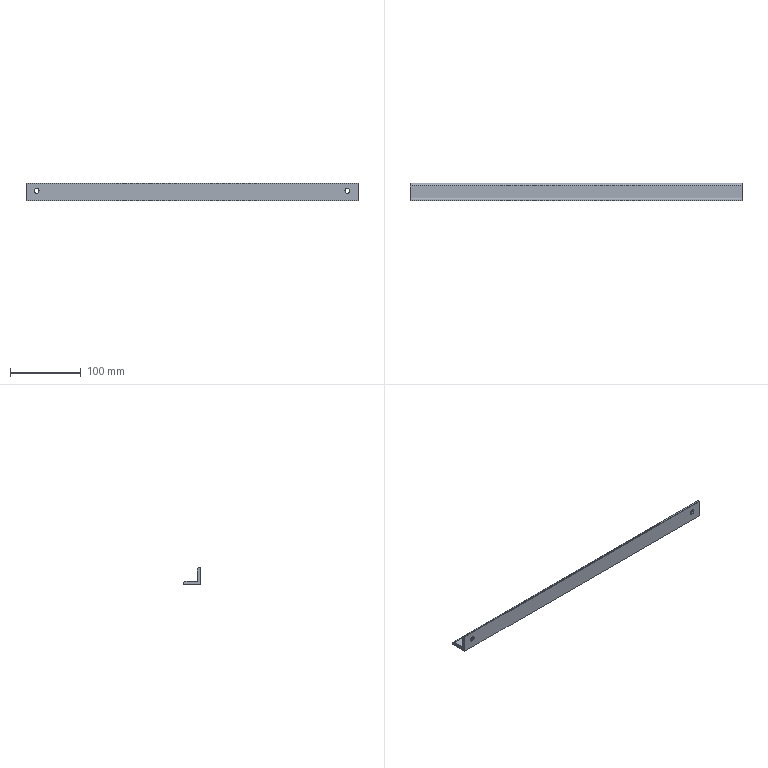Part | NX | 1 solid | 18 faces | box 470 x 25 x 25 mm | volume 101967 mm3 | plane 8 | cylinder 6 | cone 4 | commonest cylinder face diameters 7 x4 8 x2
STEP:
#1=CARTESIAN_POINT('',(-260.,12.5,-11.5));
#2=VERTEX_POINT('',#1);
#3=CARTESIAN_POINT('',(-260.,12.5,-12.5));
#4=VERTEX_POINT('',#3);
#5=CARTESIAN_POINT('',(-260.,12.5,0.));
#6=DIRECTION('',(0.,0.,-1.));
#7=VECTOR('',#6,1000.);
#8=LINE('',#5,#7);
#9=EDGE_CURVE('',#2,#4,#8,.T.);
#10=ORIENTED_EDGE('',*,*,#9,.T.);
#11=CARTESIAN_POINT('',(-260.,-12.5,-12.5));
#12=VERTEX_POINT('',#11);
#13=CARTESIAN_POINT('',(-260.,0.,-12.5));
#14=DIRECTION('',(0.,-1.,0.));
#15=VECTOR('',#14,1000.);
#16=LINE('',#13,#15);
#17=EDGE_CURVE('',#4,#12,#16,.T.);
#18=ORIENTED_EDGE('',*,*,#17,.T.);
#19=CARTESIAN_POINT('',(-260.,-12.5,12.5));
#20=VERTEX_POINT('',#19);
#21=CARTESIAN_POINT('',(-260.,-12.5,0.));
#22=DIRECTION('',(0.,0.,1.));
#23=VECTOR('',#22,1000.);
#24=LINE('',#21,#23);
#25=EDGE_CURVE('',#12,#20,#24,.T.);
#26=ORIENTED_EDGE('',*,*,#25,.T.);
#27=CARTESIAN_POINT('',(-260.,-11.5,12.5));
#28=VERTEX_POINT('',#27);
#29=CARTESIAN_POINT('',(-260.,0.,12.5));
#30=DIRECTION('',(0.,1.,0.));
#31=VECTOR('',#30,1000.);
#32=LINE('',#29,#31);
#33=EDGE_CURVE('',#20,#28,#32,.T.);
#34=ORIENTED_EDGE('',*,*,#33,.T.);
#35=CARTESIAN_POINT('',(-260.,-7.5,8.5));
#36=VERTEX_POINT('',#35);
#37=CARTESIAN_POINT('',(-260.,-11.5,8.5));
#38=DIRECTION('',(1.,0.,0.));
#39=DIRECTION('',(0.,0.,-1.));
#40=AXIS2_PLACEMENT_3D('',#37,#38,#39);
#41=CIRCLE('',#40,4.);
#42=EDGE_CURVE('',#36,#28,#41,.T.);
#43=ORIENTED_EDGE('',*,*,#42,.F.);
#44=CARTESIAN_POINT('',(-260.,-7.5,-7.5));
#45=VERTEX_POINT('',#44);
#46=CARTESIAN_POINT('',(-260.,-7.5,0.));
#47=DIRECTION('',(0.,0.,-1.));
#48=VECTOR('',#47,1000.);
#49=LINE('',#46,#48);
#50=EDGE_CURVE('',#36,#45,#49,.T.);
#51=ORIENTED_EDGE('',*,*,#50,.T.);
#52=CARTESIAN_POINT('',(-260.,8.5,-7.5));
#53=VERTEX_POINT('',#52);
#54=CARTESIAN_POINT('',(-260.,0.,-7.5));
#55=DIRECTION('',(0.,1.,0.));
#56=VECTOR('',#55,1000.);
#57=LINE('',#54,#56);
#58=EDGE_CURVE('',#45,#53,#57,.T.);
#59=ORIENTED_EDGE('',*,*,#58,.T.);
#60=CARTESIAN_POINT('',(-260.,8.5,-11.5));
#61=DIRECTION('',(1.,0.,0.));
#62=DIRECTION('',(0.,0.,-1.));
#63=AXIS2_PLACEMENT_3D('',#60,#61,#62);
#64=CIRCLE('',#63,4.);
#65=EDGE_CURVE('',#2,#53,#64,.T.);
#66=ORIENTED_EDGE('',*,*,#65,.F.);
#67=EDGE_LOOP('',(#10,#18,#26,#34,#43,#51,#59,#66));
#68=FACE_BOUND('',#67,.T.);
#69=CARTESIAN_POINT('',(-260.,0.,0.));
#70=DIRECTION('',(1.,0.,0.));
#71=DIRECTION('',(0.,1.,0.));
#72=AXIS2_PLACEMENT_3D('',#69,#70,#71);
#73=PLANE('',#72);
#74=ADVANCED_FACE('',(#68),#73,.F.);
#75=ORIENTED_EDGE('',*,*,#9,.F.);
#76=CARTESIAN_POINT('',(210.,12.5,-11.5));
#77=VERTEX_POINT('',#76);
#78=CARTESIAN_POINT('',(-260.,12.5,-11.5));
#79=DIRECTION('',(1.,0.,0.));
#80=VECTOR('',#79,1000.);
#81=LINE('',#78,#80);
#82=EDGE_CURVE('',#2,#77,#81,.T.);
#83=ORIENTED_EDGE('',*,*,#82,.T.);
#84=CARTESIAN_POINT('',(210.,12.5,-12.5));
#85=VERTEX_POINT('',#84);
#86=CARTESIAN_POINT('',(210.,12.5,0.));
#87=DIRECTION('',(0.,0.,-1.));
#88=VECTOR('',#87,1000.);
#89=LINE('',#86,#88);
#90=EDGE_CURVE('',#77,#85,#89,.T.);
#91=ORIENTED_EDGE('',*,*,#90,.T.);
#92=CARTESIAN_POINT('',(0.,12.5,-12.5));
#93=DIRECTION('',(-1.,0.,0.));
#94=VECTOR('',#93,1000.);
#95=LINE('',#92,#94);
#96=EDGE_CURVE('',#85,#4,#95,.T.);
#97=ORIENTED_EDGE('',*,*,#96,.T.);
#98=EDGE_LOOP('',(#75,#83,#91,#97));
#99=FACE_BOUND('',#98,.T.);
#100=CARTESIAN_POINT('',(-260.,12.5,-12.5));
#101=DIRECTION('',(0.,1.,0.));
#102=DIRECTION('',(1.,0.,0.));
#103=AXIS2_PLACEMENT_3D('',#100,#101,#102);
#104=PLANE('',#103);
#105=ADVANCED_FACE('',(#99),#104,.T.);
#106=ORIENTED_EDGE('',*,*,#17,.F.);
#107=ORIENTED_EDGE('',*,*,#96,.F.);
#108=CARTESIAN_POINT('',(210.,-12.5,-12.5));
#109=VERTEX_POINT('',#108);
#110=CARTESIAN_POINT('',(210.,0.,-12.5));
#111=DIRECTION('',(0.,-1.,0.));
#112=VECTOR('',#111,1000.);
#113=LINE('',#110,#112);
#114=EDGE_CURVE('',#85,#109,#113,.T.);
#115=ORIENTED_EDGE('',*,*,#114,.T.);
#116=CARTESIAN_POINT('',(0.,-12.5,-12.5));
#117=DIRECTION('',(-1.,0.,0.));
#118=VECTOR('',#117,1000.);
#119=LINE('',#116,#118);
#120=EDGE_CURVE('',#109,#12,#119,.T.);
#121=ORIENTED_EDGE('',*,*,#120,.T.);
#122=EDGE_LOOP('',(#106,#107,#115,#121));
#123=FACE_BOUND('',#122,.T.);
#124=CARTESIAN_POINT('',(-260.,-12.5,-12.5));
#125=DIRECTION('',(0.,0.,-1.));
#126=DIRECTION('',(0.,-1.,0.));
#127=AXIS2_PLACEMENT_3D('',#124,#125,#126);
#128=PLANE('',#127);
#129=ADVANCED_FACE('',(#123),#128,.T.);
#130=ORIENTED_EDGE('',*,*,#25,.F.);
#131=ORIENTED_EDGE('',*,*,#120,.F.);
#132=CARTESIAN_POINT('',(210.,-12.5,12.5));
#133=VERTEX_POINT('',#132);
#134=CARTESIAN_POINT('',(210.,-12.5,0.));
#135=DIRECTION('',(0.,0.,1.));
#136=VECTOR('',#135,1000.);
#137=LINE('',#134,#136);
#138=EDGE_CURVE('',#109,#133,#137,.T.);
#139=ORIENTED_EDGE('',*,*,#138,.T.);
#140=CARTESIAN_POINT('',(0.,-12.5,12.5));
#141=DIRECTION('',(-1.,0.,0.));
#142=VECTOR('',#141,1000.);
#143=LINE('',#140,#142);
#144=EDGE_CURVE('',#133,#20,#143,.T.);
#145=ORIENTED_EDGE('',*,*,#144,.T.);
#146=EDGE_LOOP('',(#130,#131,#139,#145));
#147=FACE_BOUND('',#146,.T.);
#148=CARTESIAN_POINT('',(-248.5,-12.5,1.5));
#149=VERTEX_POINT('',#148);
#150=CARTESIAN_POINT('',(-241.5,-12.5,1.5));
#151=VERTEX_POINT('',#150);
#152=CARTESIAN_POINT('',(-245.,-12.5,1.5));
#153=DIRECTION('',(0.,-1.,0.));
#154=DIRECTION('',(1.,0.,0.));
#155=AXIS2_PLACEMENT_3D('',#152,#153,#154);
#156=CIRCLE('',#155,3.5);
#157=EDGE_CURVE('',#149,#151,#156,.T.);
#158=ORIENTED_EDGE('',*,*,#157,.F.);
#159=CARTESIAN_POINT('',(-245.,-12.5,1.5));
#160=DIRECTION('',(0.,-1.,0.));
#161=DIRECTION('',(1.,0.,0.));
#162=AXIS2_PLACEMENT_3D('',#159,#160,#161);
#163=CIRCLE('',#162,3.5);
#164=EDGE_CURVE('',#151,#149,#163,.T.);
#165=ORIENTED_EDGE('',*,*,#164,.F.);
#166=EDGE_LOOP('',(#158,#165));
#167=FACE_BOUND('',#166,.T.);
#168=CARTESIAN_POINT('',(198.5,-12.5,1.5));
#169=VERTEX_POINT('',#168);
#170=CARTESIAN_POINT('',(191.5,-12.5,1.5));
#171=VERTEX_POINT('',#170);
#172=CARTESIAN_POINT('',(195.,-12.5,1.5));
#173=DIRECTION('',(0.,-1.,0.));
#174=DIRECTION('',(1.,0.,0.));
#175=AXIS2_PLACEMENT_3D('',#172,#173,#174);
#176=CIRCLE('',#175,3.5);
#177=EDGE_CURVE('',#169,#171,#176,.T.);
#178=ORIENTED_EDGE('',*,*,#177,.F.);
#179=CARTESIAN_POINT('',(195.,-12.5,1.5));
#180=DIRECTION('',(0.,-1.,0.));
#181=DIRECTION('',(1.,0.,0.));
#182=AXIS2_PLACEMENT_3D('',#179,#180,#181);
#183=CIRCLE('',#182,3.5);
#184=EDGE_CURVE('',#171,#169,#183,.T.);
#185=ORIENTED_EDGE('',*,*,#184,.F.);
#186=EDGE_LOOP('',(#178,#185));
#187=FACE_BOUND('',#186,.T.);
#188=CARTESIAN_POINT('',(-260.,-12.5,12.5));
#189=DIRECTION('',(0.,-1.,0.));
#190=DIRECTION('',(0.,0.,-1.));
#191=AXIS2_PLACEMENT_3D('',#188,#189,#190);
#192=PLANE('',#191);
#193=ADVANCED_FACE('',(#147,#167,#187),#192,.T.);
#194=ORIENTED_EDGE('',*,*,#33,.F.);
#195=ORIENTED_EDGE('',*,*,#144,.F.);
#196=CARTESIAN_POINT('',(210.,-11.5,12.5));
#197=VERTEX_POINT('',#196);
#198=CARTESIAN_POINT('',(210.,0.,12.5));
#199=DIRECTION('',(0.,1.,0.));
#200=VECTOR('',#199,1000.);
#201=LINE('',#198,#200);
#202=EDGE_CURVE('',#133,#197,#201,.T.);
#203=ORIENTED_EDGE('',*,*,#202,.T.);
#204=CARTESIAN_POINT('',(260.,-11.5,12.5));
#205=DIRECTION('',(-1.,0.,0.));
#206=VECTOR('',#205,1000.);
#207=LINE('',#204,#206);
#208=EDGE_CURVE('',#197,#28,#207,.T.);
#209=ORIENTED_EDGE('',*,*,#208,.T.);
#210=EDGE_LOOP('',(#194,#195,#203,#209));
#211=FACE_BOUND('',#210,.T.);
#212=CARTESIAN_POINT('',(-260.,-11.5,12.5));
#213=DIRECTION('',(0.,0.,1.));
#214=DIRECTION('',(1.,0.,0.));
#215=AXIS2_PLACEMENT_3D('',#212,#213,#214);
#216=PLANE('',#215);
#217=ADVANCED_FACE('',(#211),#216,.T.);
#218=ORIENTED_EDGE('',*,*,#42,.T.);
#219=ORIENTED_EDGE('',*,*,#208,.F.);
#220=CARTESIAN_POINT('',(210.,-7.5,8.5));
#221=VERTEX_POINT('',#220);
#222=CARTESIAN_POINT('',(210.,-11.5,8.5));
#223=DIRECTION('',(1.,0.,0.));
#224=DIRECTION('',(0.,0.,-1.));
#225=AXIS2_PLACEMENT_3D('',#222,#223,#224);
#226=CIRCLE('',#225,4.);
#227=EDGE_CURVE('',#221,#197,#226,.T.);
#228=ORIENTED_EDGE('',*,*,#227,.F.);
#229=CARTESIAN_POINT('',(-260.,-7.5,8.5));
#230=DIRECTION('',(1.,0.,0.));
#231=VECTOR('',#230,1000.);
#232=LINE('',#229,#231);
#233=EDGE_CURVE('',#36,#221,#232,.T.);
#234=ORIENTED_EDGE('',*,*,#233,.F.);
#235=EDGE_LOOP('',(#218,#219,#228,#234));
#236=FACE_BOUND('',#235,.T.);
#237=CARTESIAN_POINT('',(-260.,-11.5,8.5));
#238=DIRECTION('',(1.,0.,0.));
#239=DIRECTION('',(0.,0.,-1.));
#240=AXIS2_PLACEMENT_3D('',#237,#238,#239);
#241=CYLINDRICAL_SURFACE('',#240,4.);
#242=ADVANCED_FACE('',(#236),#241,.T.);
#243=ORIENTED_EDGE('',*,*,#50,.F.);
#244=ORIENTED_EDGE('',*,*,#233,.T.);
#245=CARTESIAN_POINT('',(210.,-7.5,-7.5));
#246=VERTEX_POINT('',#245);
#247=CARTESIAN_POINT('',(210.,-7.5,0.));
#248=DIRECTION('',(0.,0.,-1.));
#249=VECTOR('',#248,1000.);
#250=LINE('',#247,#249);
#251=EDGE_CURVE('',#221,#246,#250,.T.);
#252=ORIENTED_EDGE('',*,*,#251,.T.);
#253=CARTESIAN_POINT('',(0.,-7.5,-7.5));
#254=DIRECTION('',(-1.,0.,0.));
#255=VECTOR('',#254,1000.);
#256=LINE('',#253,#255);
#257=EDGE_CURVE('',#246,#45,#256,.T.);
#258=ORIENTED_EDGE('',*,*,#257,.T.);
#259=EDGE_LOOP('',(#243,#244,#252,#258));
#260=FACE_BOUND('',#259,.T.);
#261=CARTESIAN_POINT('',(-239.,-7.5,1.5));
#262=VERTEX_POINT('',#261);
#263=CARTESIAN_POINT('',(-251.,-7.5,1.5));
#264=VERTEX_POINT('',#263);
#265=CARTESIAN_POINT('',(-245.,-7.5,1.5));
#266=DIRECTION('',(0.,1.,0.));
#267=DIRECTION('',(-1.,0.,0.));
#268=AXIS2_PLACEMENT_3D('',#265,#266,#267);
#269=CIRCLE('',#268,6.);
#270=EDGE_CURVE('',#262,#264,#269,.T.);
#271=ORIENTED_EDGE('',*,*,#270,.F.);
#272=CARTESIAN_POINT('',(-245.,-7.5,1.5));
#273=DIRECTION('',(0.,1.,0.));
#274=DIRECTION('',(-1.,0.,0.));
#275=AXIS2_PLACEMENT_3D('',#272,#273,#274);
#276=CIRCLE('',#275,6.);
#277=EDGE_CURVE('',#264,#262,#276,.T.);
#278=ORIENTED_EDGE('',*,*,#277,.F.);
#279=EDGE_LOOP('',(#271,#278));
#280=FACE_BOUND('',#279,.T.);
#281=CARTESIAN_POINT('',(189.,-7.5,1.5));
#282=VERTEX_POINT('',#281);
#283=CARTESIAN_POINT('',(201.,-7.5,1.5));
#284=VERTEX_POINT('',#283);
#285=CARTESIAN_POINT('',(195.,-7.5,1.5));
#286=DIRECTION('',(0.,1.,0.));
#287=DIRECTION('',(-1.,0.,0.));
#288=AXIS2_PLACEMENT_3D('',#285,#286,#287);
#289=CIRCLE('',#288,6.);
#290=EDGE_CURVE('',#282,#284,#289,.T.);
#291=ORIENTED_EDGE('',*,*,#290,.F.);
#292=CARTESIAN_POINT('',(195.,-7.5,1.5));
#293=DIRECTION('',(0.,1.,0.));
#294=DIRECTION('',(-1.,0.,0.));
#295=AXIS2_PLACEMENT_3D('',#292,#293,#294);
#296=CIRCLE('',#295,6.);
#297=EDGE_CURVE('',#284,#282,#296,.T.);
#298=ORIENTED_EDGE('',*,*,#297,.F.);
#299=EDGE_LOOP('',(#291,#298));
#300=FACE_BOUND('',#299,.T.);
#301=CARTESIAN_POINT('',(-260.,-7.5,-7.5));
#302=DIRECTION('',(0.,1.,0.));
#303=DIRECTION('',(1.,0.,0.));
#304=AXIS2_PLACEMENT_3D('',#301,#302,#303);
#305=PLANE('',#304);
#306=ADVANCED_FACE('',(#260,#280,#300),#305,.T.);
#307=ORIENTED_EDGE('',*,*,#58,.F.);
#308=ORIENTED_EDGE('',*,*,#257,.F.);
#309=CARTESIAN_POINT('',(210.,8.5,-7.5));
#310=VERTEX_POINT('',#309);
#311=CARTESIAN_POINT('',(210.,0.,-7.5));
#312=DIRECTION('',(0.,1.,0.));
#313=VECTOR('',#312,1000.);
#314=LINE('',#311,#313);
#315=EDGE_CURVE('',#246,#310,#314,.T.);
#316=ORIENTED_EDGE('',*,*,#315,.T.);
#317=CARTESIAN_POINT('',(260.,8.5,-7.5));
#318=DIRECTION('',(-1.,0.,0.));
#319=VECTOR('',#318,1000.);
#320=LINE('',#317,#319);
#321=EDGE_CURVE('',#310,#53,#320,.T.);
#322=ORIENTED_EDGE('',*,*,#321,.T.);
#323=EDGE_LOOP('',(#307,#308,#316,#322));
#324=FACE_BOUND('',#323,.T.);
#325=CARTESIAN_POINT('',(-260.,8.5,-7.5));
#326=DIRECTION('',(0.,0.,1.));
#327=DIRECTION('',(1.,0.,0.));
#328=AXIS2_PLACEMENT_3D('',#325,#326,#327);
#329=PLANE('',#328);
#330=ADVANCED_FACE('',(#324),#329,.T.);
#331=ORIENTED_EDGE('',*,*,#65,.T.);
#332=ORIENTED_EDGE('',*,*,#321,.F.);
#333=CARTESIAN_POINT('',(210.,8.5,-11.5));
#334=DIRECTION('',(1.,0.,0.));
#335=DIRECTION('',(0.,0.,-1.));
#336=AXIS2_PLACEMENT_3D('',#333,#334,#335);
#337=CIRCLE('',#336,4.);
#338=EDGE_CURVE('',#77,#310,#337,.T.);
#339=ORIENTED_EDGE('',*,*,#338,.F.);
#340=ORIENTED_EDGE('',*,*,#82,.F.);
#341=EDGE_LOOP('',(#331,#332,#339,#340));
#342=FACE_BOUND('',#341,.T.);
#343=CARTESIAN_POINT('',(-260.,8.5,-11.5));
#344=DIRECTION('',(1.,0.,0.));
#345=DIRECTION('',(0.,0.,-1.));
#346=AXIS2_PLACEMENT_3D('',#343,#344,#345);
#347=CYLINDRICAL_SURFACE('',#346,4.);
#348=ADVANCED_FACE('',(#342),#347,.T.);
#349=ORIENTED_EDGE('',*,*,#90,.F.);
#350=ORIENTED_EDGE('',*,*,#338,.T.);
#351=ORIENTED_EDGE('',*,*,#315,.F.);
#352=ORIENTED_EDGE('',*,*,#251,.F.);
#353=ORIENTED_EDGE('',*,*,#227,.T.);
#354=ORIENTED_EDGE('',*,*,#202,.F.);
#355=ORIENTED_EDGE('',*,*,#138,.F.);
#356=ORIENTED_EDGE('',*,*,#114,.F.);
#357=EDGE_LOOP('',(#349,#350,#351,#352,#353,#354,#355,#356));
#358=FACE_BOUND('',#357,.T.);
#359=CARTESIAN_POINT('',(210.,0.,0.));
#360=DIRECTION('',(1.,0.,0.));
#361=DIRECTION('',(0.,1.,0.));
#362=AXIS2_PLACEMENT_3D('',#359,#360,#361);
#363=PLANE('',#362);
#364=ADVANCED_FACE('',(#358),#363,.T.);
#365=CARTESIAN_POINT('',(-248.5,-10.,1.5));
#366=VERTEX_POINT('',#365);
#367=CARTESIAN_POINT('',(-241.5,-10.,1.5));
#368=VERTEX_POINT('',#367);
#369=CARTESIAN_POINT('',(-245.,-10.,1.5));
#370=DIRECTION('',(0.,1.,0.));
#371=DIRECTION('',(-1.,0.,0.));
#372=AXIS2_PLACEMENT_3D('',#369,#370,#371);
#373=CIRCLE('',#372,3.5);
#374=EDGE_CURVE('',#366,#368,#373,.T.);
#375=ORIENTED_EDGE('',*,*,#374,.F.);
#376=CARTESIAN_POINT('',(-249.75,-8.75,1.5));
#377=DIRECTION('',(-0.7071,0.7071,0.));
#378=VECTOR('',#377,1000.);
#379=LINE('',#376,#378);
#380=EDGE_CURVE('',#264,#366,#379,.F.);
#381=ORIENTED_EDGE('',*,*,#380,.F.);
#382=ORIENTED_EDGE('',*,*,#277,.T.);
#383=CARTESIAN_POINT('',(-240.25,-8.75,1.5));
#384=DIRECTION('',(0.7071,0.7071,0.));
#385=VECTOR('',#384,1000.);
#386=LINE('',#383,#385);
#387=EDGE_CURVE('',#262,#368,#386,.F.);
#388=ORIENTED_EDGE('',*,*,#387,.T.);
#389=EDGE_LOOP('',(#375,#381,#382,#388));
#390=FACE_BOUND('',#389,.T.);
#391=CARTESIAN_POINT('',(-245.,-8.75,1.5));
#392=DIRECTION('',(0.,1.,0.));
#393=DIRECTION('',(1.,0.,0.));
#394=AXIS2_PLACEMENT_3D('',#391,#392,#393);
#395=CONICAL_SURFACE('',#394,4.75,0.7854);
#396=ADVANCED_FACE('',(#390),#395,.F.);
#397=ORIENTED_EDGE('',*,*,#290,.T.);
#398=CARTESIAN_POINT('',(198.5,-10.,1.5));
#399=VERTEX_POINT('',#398);
#400=CARTESIAN_POINT('',(199.75,-8.75,1.5));
#401=DIRECTION('',(0.7071,0.7071,0.));
#402=VECTOR('',#401,1000.);
#403=LINE('',#400,#402);
#404=EDGE_CURVE('',#399,#284,#403,.T.);
#405=ORIENTED_EDGE('',*,*,#404,.F.);
#406=CARTESIAN_POINT('',(191.5,-10.,1.5));
#407=VERTEX_POINT('',#406);
#408=CARTESIAN_POINT('',(195.,-10.,1.5));
#409=DIRECTION('',(0.,1.,0.));
#410=DIRECTION('',(-1.,0.,0.));
#411=AXIS2_PLACEMENT_3D('',#408,#409,#410);
#412=CIRCLE('',#411,3.5);
#413=EDGE_CURVE('',#407,#399,#412,.T.);
#414=ORIENTED_EDGE('',*,*,#413,.F.);
#415=CARTESIAN_POINT('',(190.25,-8.75,1.5));
#416=DIRECTION('',(-0.7071,0.7071,0.));
#417=VECTOR('',#416,1000.);
#418=LINE('',#415,#417);
#419=EDGE_CURVE('',#407,#282,#418,.T.);
#420=ORIENTED_EDGE('',*,*,#419,.T.);
#421=EDGE_LOOP('',(#397,#405,#414,#420));
#422=FACE_BOUND('',#421,.T.);
#423=CARTESIAN_POINT('',(195.,-8.75,1.5));
#424=DIRECTION('',(0.,1.,0.));
#425=DIRECTION('',(1.,0.,0.));
#426=AXIS2_PLACEMENT_3D('',#423,#424,#425);
#427=CONICAL_SURFACE('',#426,4.75,0.7854);
#428=ADVANCED_FACE('',(#422),#427,.F.);
#429=ORIENTED_EDGE('',*,*,#374,.T.);
#430=CARTESIAN_POINT('',(-241.5,-31.125,1.5));
#431=DIRECTION('',(0.,1.,0.));
#432=VECTOR('',#431,1000.);
#433=LINE('',#430,#432);
#434=EDGE_CURVE('',#151,#368,#433,.T.);
#435=ORIENTED_EDGE('',*,*,#434,.F.);
#436=ORIENTED_EDGE('',*,*,#164,.T.);
#437=CARTESIAN_POINT('',(-248.5,-31.125,1.5));
#438=DIRECTION('',(0.,1.,0.));
#439=VECTOR('',#438,1000.);
#440=LINE('',#437,#439);
#441=EDGE_CURVE('',#149,#366,#440,.T.);
#442=ORIENTED_EDGE('',*,*,#441,.T.);
#443=EDGE_LOOP('',(#429,#435,#436,#442));
#444=FACE_BOUND('',#443,.T.);
#445=CARTESIAN_POINT('',(-245.,-31.125,1.5));
#446=DIRECTION('',(0.,1.,0.));
#447=DIRECTION('',(1.,0.,0.));
#448=AXIS2_PLACEMENT_3D('',#445,#446,#447);
#449=CYLINDRICAL_SURFACE('',#448,3.5);
#450=ADVANCED_FACE('',(#444),#449,.F.);
#451=ORIENTED_EDGE('',*,*,#177,.T.);
#452=CARTESIAN_POINT('',(191.5,-31.125,1.5));
#453=DIRECTION('',(0.,1.,0.));
#454=VECTOR('',#453,1000.);
#455=LINE('',#452,#454);
#456=EDGE_CURVE('',#171,#407,#455,.T.);
#457=ORIENTED_EDGE('',*,*,#456,.T.);
#458=ORIENTED_EDGE('',*,*,#413,.T.);
#459=CARTESIAN_POINT('',(198.5,-31.125,1.5));
#460=DIRECTION('',(0.,1.,0.));
#461=VECTOR('',#460,1000.);
#462=LINE('',#459,#461);
#463=EDGE_CURVE('',#169,#399,#462,.T.);
#464=ORIENTED_EDGE('',*,*,#463,.F.);
#465=EDGE_LOOP('',(#451,#457,#458,#464));
#466=FACE_BOUND('',#465,.T.);
#467=CARTESIAN_POINT('',(195.,-31.125,1.5));
#468=DIRECTION('',(0.,1.,0.));
#469=DIRECTION('',(1.,0.,0.));
#470=AXIS2_PLACEMENT_3D('',#467,#468,#469);
#471=CYLINDRICAL_SURFACE('',#470,3.5);
#472=ADVANCED_FACE('',(#466),#471,.F.);
#473=ORIENTED_EDGE('',*,*,#463,.T.);
#474=CARTESIAN_POINT('',(195.,-10.,1.5));
#475=DIRECTION('',(0.,1.,0.));
#476=DIRECTION('',(-1.,0.,0.));
#477=AXIS2_PLACEMENT_3D('',#474,#475,#476);
#478=CIRCLE('',#477,3.5);
#479=EDGE_CURVE('',#399,#407,#478,.T.);
#480=ORIENTED_EDGE('',*,*,#479,.T.);
#481=ORIENTED_EDGE('',*,*,#456,.F.);
#482=ORIENTED_EDGE('',*,*,#184,.T.);
#483=EDGE_LOOP('',(#473,#480,#481,#482));
#484=FACE_BOUND('',#483,.T.);
#485=CARTESIAN_POINT('',(195.,-31.125,1.5));
#486=DIRECTION('',(0.,1.,0.));
#487=DIRECTION('',(1.,0.,0.));
#488=AXIS2_PLACEMENT_3D('',#485,#486,#487);
#489=CYLINDRICAL_SURFACE('',#488,3.5);
#490=ADVANCED_FACE('',(#484),#489,.F.);
#491=ORIENTED_EDGE('',*,*,#404,.T.);
#492=ORIENTED_EDGE('',*,*,#297,.T.);
#493=ORIENTED_EDGE('',*,*,#419,.F.);
#494=ORIENTED_EDGE('',*,*,#479,.F.);
#495=EDGE_LOOP('',(#491,#492,#493,#494));
#496=FACE_BOUND('',#495,.T.);
#497=CARTESIAN_POINT('',(195.,-8.75,1.5));
#498=DIRECTION('',(0.,1.,0.));
#499=DIRECTION('',(1.,0.,0.));
#500=AXIS2_PLACEMENT_3D('',#497,#498,#499);
#501=CONICAL_SURFACE('',#500,4.75,0.7854);
#502=ADVANCED_FACE('',(#496),#501,.F.);
#503=ORIENTED_EDGE('',*,*,#270,.T.);
#504=ORIENTED_EDGE('',*,*,#380,.T.);
#505=CARTESIAN_POINT('',(-245.,-10.,1.5));
#506=DIRECTION('',(0.,1.,0.));
#507=DIRECTION('',(-1.,0.,0.));
#508=AXIS2_PLACEMENT_3D('',#505,#506,#507);
#509=CIRCLE('',#508,3.5);
#510=EDGE_CURVE('',#368,#366,#509,.T.);
#511=ORIENTED_EDGE('',*,*,#510,.F.);
#512=ORIENTED_EDGE('',*,*,#387,.F.);
#513=EDGE_LOOP('',(#503,#504,#511,#512));
#514=FACE_BOUND('',#513,.T.);
#515=CARTESIAN_POINT('',(-245.,-8.75,1.5));
#516=DIRECTION('',(0.,1.,0.));
#517=DIRECTION('',(1.,0.,0.));
#518=AXIS2_PLACEMENT_3D('',#515,#516,#517);
#519=CONICAL_SURFACE('',#518,4.75,0.7854);
#520=ADVANCED_FACE('',(#514),#519,.F.);
#521=ORIENTED_EDGE('',*,*,#157,.T.);
#522=ORIENTED_EDGE('',*,*,#434,.T.);
#523=ORIENTED_EDGE('',*,*,#510,.T.);
#524=ORIENTED_EDGE('',*,*,#441,.F.);
#525=EDGE_LOOP('',(#521,#522,#523,#524));
#526=FACE_BOUND('',#525,.T.);
#527=CARTESIAN_POINT('',(-245.,-31.125,1.5));
#528=DIRECTION('',(0.,1.,0.));
#529=DIRECTION('',(1.,0.,0.));
#530=AXIS2_PLACEMENT_3D('',#527,#528,#529);
#531=CYLINDRICAL_SURFACE('',#530,3.5);
#532=ADVANCED_FACE('',(#526),#531,.F.);
#533=CLOSED_SHELL('',(#74,#105,#129,#193,#217,#242,#306,#330,#348,#364,#396,#428,#450,#472,#490,#502,#520,#532));
#534=MANIFOLD_SOLID_BREP('',#533);
#535=(LENGTH_UNIT()NAMED_UNIT(*)SI_UNIT(.MILLI.,.METRE.));
#536=UNCERTAINTY_MEASURE_WITH_UNIT(LENGTH_MEASURE(0.00001),#535,'','');
#537=(NAMED_UNIT(*)PLANE_ANGLE_UNIT()SI_UNIT($,.RADIAN.));
#538=(NAMED_UNIT(*)SI_UNIT($,.STERADIAN.)SOLID_ANGLE_UNIT());
#539=(GEOMETRIC_REPRESENTATION_CONTEXT(3)GLOBAL_UNCERTAINTY_ASSIGNED_CONTEXT((#536))GLOBAL_UNIT_ASSIGNED_CONTEXT((#535,#537,#538))REPRESENTATION_CONTEXT('',''));
#540=ADVANCED_BREP_SHAPE_REPRESENTATION('',(#534),#539);